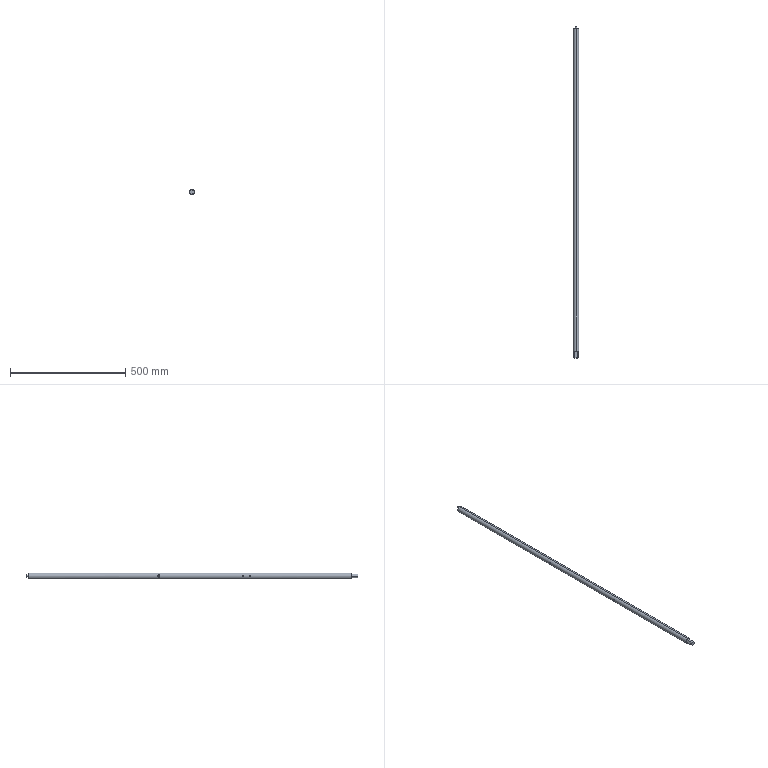Part | SolidWorks | features BaseBody 1 | 1 solid | 29 faces | box 25 x 1442 x 25 mm | volume 693874 mm3 | plane 16 | cylinder 13 | commonest cylinder face diameters 6 x9 10 x2 25 x2
STEP:
#1=CARTESIAN_POINT('',(933.402,-3520.973,899.971));
#2=VERTEX_POINT('',#1);
#3=CARTESIAN_POINT('',(933.402,-3520.973,889.971));
#4=VERTEX_POINT('',#3);
#5=CARTESIAN_POINT('',(933.402,-3520.973,899.971));
#6=CARTESIAN_POINT('',(933.402,-3520.643,899.971));
#7=CARTESIAN_POINT('',(933.417,-3520.308,899.938));
#8=CARTESIAN_POINT('',(933.472,-3519.665,899.808));
#9=CARTESIAN_POINT('',(933.512,-3519.351,899.712));
#10=CARTESIAN_POINT('',(933.613,-3518.743,899.458));
#11=CARTESIAN_POINT('',(933.672,-3518.457,899.304));
#12=CARTESIAN_POINT('',(933.799,-3517.919,898.944));
#13=CARTESIAN_POINT('',(933.868,-3517.665,898.735));
#14=CARTESIAN_POINT('',(934.003,-3517.208,898.277));
#15=CARTESIAN_POINT('',(934.069,-3517.003,898.029));
#16=CARTESIAN_POINT('',(934.193,-3516.641,897.489));
#17=CARTESIAN_POINT('',(934.249,-3516.484,897.198));
#18=CARTESIAN_POINT('',(934.343,-3516.234,896.597));
#19=CARTESIAN_POINT('',(934.381,-3516.137,896.285));
#20=CARTESIAN_POINT('',(934.432,-3516.006,895.634));
#21=CARTESIAN_POINT('',(934.446,-3515.973,895.302));
#22=CARTESIAN_POINT('',(934.445,-3515.973,894.635));
#23=CARTESIAN_POINT('',(934.432,-3516.007,894.307));
#24=CARTESIAN_POINT('',(934.381,-3516.136,893.664));
#25=CARTESIAN_POINT('',(934.343,-3516.234,893.345));
#26=CARTESIAN_POINT('',(934.249,-3516.486,892.741));
#27=CARTESIAN_POINT('',(934.193,-3516.64,892.455));
#28=CARTESIAN_POINT('',(934.069,-3517.003,891.915));
#29=CARTESIAN_POINT('',(934.002,-3517.211,891.662));
#30=CARTESIAN_POINT('',(933.867,-3517.667,891.206));
#31=CARTESIAN_POINT('',(933.8,-3517.917,891.));
#32=CARTESIAN_POINT('',(933.671,-3518.46,890.637));
#33=CARTESIAN_POINT('',(933.613,-3518.745,890.483));
#34=CARTESIAN_POINT('',(933.538,-3519.195,890.295));
#35=CARTESIAN_POINT('',(933.516,-3519.348,890.24));
#36=CARTESIAN_POINT('',(933.476,-3519.663,890.143));
#37=CARTESIAN_POINT('',(933.458,-3519.824,890.102));
#38=CARTESIAN_POINT('',(933.417,-3520.31,890.005));
#39=CARTESIAN_POINT('',(933.402,-3520.639,889.971));
#40=CARTESIAN_POINT('',(933.402,-3520.973,889.971));
#41=B_SPLINE_CURVE_WITH_KNOTS('',3,(#5,#6,#7,#8,#9,#10,#11,#12,#13,#14,#15,#16,#17,#18,#19,#20,#21,#22,#23,#24,#25,#26,#27,#28,#29,#30,#31,#32,#33,#34,#35,#36,#37,#38,#39,#40),.UNSPECIFIED.,.F.,.F.,(4,2,2,2,2,2,2,2,2,2,2,2,2,2,2,2,2,4),(0.02369,0.02468,0.02567,0.02665,0.02764,0.02863,0.02961,0.0306,0.03158,0.03257,0.03356,0.03454,0.03553,0.03652,0.0375,0.038,0.03849,0.03948),.UNSPECIFIED.);
#42=EDGE_CURVE('',#2,#4,#41,.T.);
#43=ORIENTED_EDGE('',*,*,#42,.T.);
#44=CARTESIAN_POINT('',(933.402,-3520.973,889.971));
#45=CARTESIAN_POINT('',(933.402,-3521.307,889.971));
#46=CARTESIAN_POINT('',(933.417,-3521.635,890.005));
#47=CARTESIAN_POINT('',(933.472,-3522.279,890.134));
#48=CARTESIAN_POINT('',(933.513,-3522.598,890.231));
#49=CARTESIAN_POINT('',(933.613,-3523.201,890.483));
#50=CARTESIAN_POINT('',(933.672,-3523.487,890.637));
#51=CARTESIAN_POINT('',(933.799,-3524.028,891.));
#52=CARTESIAN_POINT('',(933.868,-3524.28,891.208));
#53=CARTESIAN_POINT('',(934.002,-3524.737,891.664));
#54=CARTESIAN_POINT('',(934.069,-3524.943,891.914));
#55=CARTESIAN_POINT('',(934.193,-3525.308,892.458));
#56=CARTESIAN_POINT('',(934.249,-3525.461,892.744));
#57=CARTESIAN_POINT('',(934.32,-3525.649,893.194));
#58=CARTESIAN_POINT('',(934.341,-3525.705,893.348));
#59=CARTESIAN_POINT('',(934.378,-3525.802,893.663));
#60=CARTESIAN_POINT('',(934.394,-3525.843,893.825));
#61=CARTESIAN_POINT('',(934.432,-3525.94,894.312));
#62=CARTESIAN_POINT('',(934.446,-3525.973,894.641));
#63=CARTESIAN_POINT('',(934.445,-3525.973,895.309));
#64=CARTESIAN_POINT('',(934.432,-3525.939,895.637));
#65=CARTESIAN_POINT('',(934.381,-3525.81,896.281));
#66=CARTESIAN_POINT('',(934.343,-3525.712,896.6));
#67=CARTESIAN_POINT('',(934.248,-3525.459,897.204));
#68=CARTESIAN_POINT('',(934.192,-3525.305,897.49));
#69=CARTESIAN_POINT('',(934.069,-3524.941,898.031));
#70=CARTESIAN_POINT('',(934.001,-3524.732,898.284));
#71=CARTESIAN_POINT('',(933.867,-3524.276,898.739));
#72=CARTESIAN_POINT('',(933.799,-3524.025,898.945));
#73=CARTESIAN_POINT('',(933.67,-3523.482,899.309));
#74=CARTESIAN_POINT('',(933.612,-3523.196,899.462));
#75=CARTESIAN_POINT('',(933.537,-3522.746,899.65));
#76=CARTESIAN_POINT('',(933.515,-3522.592,899.705));
#77=CARTESIAN_POINT('',(933.475,-3522.277,899.801));
#78=CARTESIAN_POINT('',(933.458,-3522.115,899.842));
#79=CARTESIAN_POINT('',(933.416,-3521.63,899.939));
#80=CARTESIAN_POINT('',(933.402,-3521.303,899.971));
#81=CARTESIAN_POINT('',(933.402,-3520.973,899.971));
#82=B_SPLINE_CURVE_WITH_KNOTS('',3,(#44,#45,#46,#47,#48,#49,#50,#51,#52,#53,#54,#55,#56,#57,#58,#59,#60,#61,#62,#63,#64,#65,#66,#67,#68,#69,#70,#71,#72,#73,#74,#75,#76,#77,#78,#79,#80,#81),.UNSPECIFIED.,.F.,.F.,(4,2,2,2,2,2,2,2,2,2,2,2,2,2,2,2,2,2,4),(0.007895,0.008882,0.00987,0.01086,0.01184,0.01283,0.01382,0.01431,0.01481,0.01579,0.01678,0.01777,0.01876,0.01974,0.02073,0.02172,0.02221,0.02271,0.02369),.UNSPECIFIED.);
#83=EDGE_CURVE('',#4,#2,#82,.T.);
#84=ORIENTED_EDGE('',*,*,#83,.T.);
#85=EDGE_LOOP('',(#43,#84));
#86=FACE_BOUND('',#85,.T.);
#87=CARTESIAN_POINT('',(921.946,-2953.973,882.471));
#88=VERTEX_POINT('',#87);
#89=CARTESIAN_POINT('',(921.946,-2953.973,907.471));
#90=VERTEX_POINT('',#89);
#91=CARTESIAN_POINT('',(921.946,-2953.973,894.971));
#92=DIRECTION('',(0.,-1.,0.));
#93=DIRECTION('',(0.,0.,-1.));
#94=AXIS2_PLACEMENT_3D('',#91,#92,#93);
#95=CIRCLE('',#94,12.5);
#96=EDGE_CURVE('',#88,#90,#95,.T.);
#97=ORIENTED_EDGE('',*,*,#96,.T.);
#98=CARTESIAN_POINT('',(921.946,-4355.973,907.471));
#99=VERTEX_POINT('',#98);
#100=CARTESIAN_POINT('',(921.946,-3669.973,907.471));
#101=DIRECTION('',(0.,-1.,0.));
#102=VECTOR('',#101,1000.);
#103=LINE('',#100,#102);
#104=EDGE_CURVE('',#90,#99,#103,.T.);
#105=ORIENTED_EDGE('',*,*,#104,.T.);
#106=CARTESIAN_POINT('',(921.946,-4355.973,882.471));
#107=VERTEX_POINT('',#106);
#108=CARTESIAN_POINT('',(921.946,-4355.973,894.971));
#109=DIRECTION('',(0.,1.,0.));
#110=DIRECTION('',(0.,0.,-1.));
#111=AXIS2_PLACEMENT_3D('',#108,#109,#110);
#112=CIRCLE('',#111,12.5);
#113=EDGE_CURVE('',#99,#107,#112,.T.);
#114=ORIENTED_EDGE('',*,*,#113,.T.);
#115=CARTESIAN_POINT('',(921.946,-3669.973,882.471));
#116=DIRECTION('',(0.,-1.,0.));
#117=VECTOR('',#116,1000.);
#118=LINE('',#115,#117);
#119=EDGE_CURVE('',#88,#107,#118,.T.);
#120=ORIENTED_EDGE('',*,*,#119,.F.);
#121=EDGE_LOOP('',(#97,#105,#114,#120));
#122=FACE_OUTER_BOUND('',#121,.T.);
#123=CARTESIAN_POINT('',(921.946,-3669.973,894.971));
#124=DIRECTION('',(0.,-1.,0.));
#125=DIRECTION('',(0.,0.,-1.));
#126=AXIS2_PLACEMENT_3D('',#123,#124,#125);
#127=CYLINDRICAL_SURFACE('',#126,12.5);
#128=ADVANCED_FACE('',(#86,#122),#127,.T.);
#129=ORIENTED_EDGE('',*,*,#83,.F.);
#130=CARTESIAN_POINT('',(910.489,-3520.973,889.971));
#131=VERTEX_POINT('',#130);
#132=CARTESIAN_POINT('',(921.679,-3520.973,889.971));
#133=DIRECTION('',(-1.,0.,0.));
#134=VECTOR('',#133,1000.);
#135=LINE('',#132,#134);
#136=EDGE_CURVE('',#4,#131,#135,.T.);
#137=ORIENTED_EDGE('',*,*,#136,.T.);
#138=CARTESIAN_POINT('',(910.489,-3520.973,899.971));
#139=VERTEX_POINT('',#138);
#140=CARTESIAN_POINT('',(910.489,-3520.973,899.971));
#141=CARTESIAN_POINT('',(910.489,-3521.303,899.971));
#142=CARTESIAN_POINT('',(910.474,-3521.638,899.938));
#143=CARTESIAN_POINT('',(910.419,-3522.282,899.808));
#144=CARTESIAN_POINT('',(910.379,-3522.595,899.712));
#145=CARTESIAN_POINT('',(910.278,-3523.204,899.458));
#146=CARTESIAN_POINT('',(910.219,-3523.489,899.304));
#147=CARTESIAN_POINT('',(910.092,-3524.027,898.944));
#148=CARTESIAN_POINT('',(910.023,-3524.281,898.735));
#149=CARTESIAN_POINT('',(909.888,-3524.738,898.277));
#150=CARTESIAN_POINT('',(909.822,-3524.943,898.029));
#151=CARTESIAN_POINT('',(909.699,-3525.305,897.489));
#152=CARTESIAN_POINT('',(909.642,-3525.462,897.198));
#153=CARTESIAN_POINT('',(909.548,-3525.713,896.597));
#154=CARTESIAN_POINT('',(909.51,-3525.809,896.285));
#155=CARTESIAN_POINT('',(909.459,-3525.94,895.634));
#156=CARTESIAN_POINT('',(909.445,-3525.973,895.302));
#157=CARTESIAN_POINT('',(909.446,-3525.973,894.635));
#158=CARTESIAN_POINT('',(909.459,-3525.94,894.307));
#159=CARTESIAN_POINT('',(909.51,-3525.81,893.664));
#160=CARTESIAN_POINT('',(909.548,-3525.712,893.345));
#161=CARTESIAN_POINT('',(909.642,-3525.46,892.741));
#162=CARTESIAN_POINT('',(909.698,-3525.306,892.455));
#163=CARTESIAN_POINT('',(909.822,-3524.943,891.915));
#164=CARTESIAN_POINT('',(909.889,-3524.735,891.662));
#165=CARTESIAN_POINT('',(910.024,-3524.279,891.206));
#166=CARTESIAN_POINT('',(910.092,-3524.029,891.));
#167=CARTESIAN_POINT('',(910.22,-3523.486,890.637));
#168=CARTESIAN_POINT('',(910.278,-3523.201,890.483));
#169=CARTESIAN_POINT('',(910.353,-3522.751,890.295));
#170=CARTESIAN_POINT('',(910.376,-3522.598,890.24));
#171=CARTESIAN_POINT('',(910.415,-3522.283,890.143));
#172=CARTESIAN_POINT('',(910.433,-3522.122,890.102));
#173=CARTESIAN_POINT('',(910.474,-3521.636,890.005));
#174=CARTESIAN_POINT('',(910.489,-3521.307,889.971));
#175=CARTESIAN_POINT('',(910.489,-3520.973,889.971));
#176=B_SPLINE_CURVE_WITH_KNOTS('',3,(#140,#141,#142,#143,#144,#145,#146,#147,#148,#149,#150,#151,#152,#153,#154,#155,#156,#157,#158,#159,#160,#161,#162,#163,#164,#165,#166,#167,#168,#169,#170,#171,#172,#173,#174,#175),.UNSPECIFIED.,.F.,.F.,(4,2,2,2,2,2,2,2,2,2,2,2,2,2,2,2,2,4),(0.02369,0.02468,0.02567,0.02665,0.02764,0.02863,0.02961,0.0306,0.03158,0.03257,0.03356,0.03454,0.03553,0.03652,0.0375,0.038,0.03849,0.03948),.UNSPECIFIED.);
#177=EDGE_CURVE('',#139,#131,#176,.T.);
#178=ORIENTED_EDGE('',*,*,#177,.F.);
#179=CARTESIAN_POINT('',(921.679,-3520.973,899.971));
#180=DIRECTION('',(-1.,0.,0.));
#181=VECTOR('',#180,1000.);
#182=LINE('',#179,#181);
#183=EDGE_CURVE('',#2,#139,#182,.T.);
#184=ORIENTED_EDGE('',*,*,#183,.F.);
#185=EDGE_LOOP('',(#129,#137,#178,#184));
#186=FACE_OUTER_BOUND('',#185,.T.);
#187=CARTESIAN_POINT('',(921.679,-3520.973,894.971));
#188=DIRECTION('',(-1.,0.,0.));
#189=DIRECTION('',(0.,0.,1.));
#190=AXIS2_PLACEMENT_3D('',#187,#188,#189);
#191=CYLINDRICAL_SURFACE('',#190,5.);
#192=ADVANCED_FACE('',(#186),#191,.F.);
#193=CARTESIAN_POINT('',(916.446,-3885.973,892.044));
#194=VERTEX_POINT('',#193);
#195=CARTESIAN_POINT('',(916.446,-3885.973,898.044));
#196=VERTEX_POINT('',#195);
#197=CARTESIAN_POINT('',(916.446,-3885.973,895.044));
#198=DIRECTION('',(-1.,0.,0.));
#199=DIRECTION('',(0.,0.,1.));
#200=AXIS2_PLACEMENT_3D('',#197,#198,#199);
#201=CIRCLE('',#200,3.);
#202=EDGE_CURVE('',#194,#196,#201,.T.);
#203=ORIENTED_EDGE('',*,*,#202,.F.);
#204=CARTESIAN_POINT('',(909.793,-3885.973,892.044));
#205=VERTEX_POINT('',#204);
#206=CARTESIAN_POINT('',(866.446,-3885.973,892.044));
#207=DIRECTION('',(-1.,0.,0.));
#208=VECTOR('',#207,1000.);
#209=LINE('',#206,#208);
#210=EDGE_CURVE('',#194,#205,#209,.T.);
#211=ORIENTED_EDGE('',*,*,#210,.T.);
#212=CARTESIAN_POINT('',(909.829,-3885.973,898.044));
#213=VERTEX_POINT('',#212);
#214=CARTESIAN_POINT('',(909.829,-3885.973,898.044));
#215=CARTESIAN_POINT('',(909.829,-3886.169,898.044));
#216=CARTESIAN_POINT('',(909.824,-3886.369,898.024));
#217=CARTESIAN_POINT('',(909.805,-3886.754,897.947));
#218=CARTESIAN_POINT('',(909.791,-3886.941,897.89));
#219=CARTESIAN_POINT('',(909.738,-3887.487,897.664));
#220=CARTESIAN_POINT('',(909.689,-3887.816,897.443));
#221=CARTESIAN_POINT('',(909.615,-3888.233,897.027));
#222=CARTESIAN_POINT('',(909.59,-3888.356,896.877));
#223=CARTESIAN_POINT('',(909.545,-3888.573,896.553));
#224=CARTESIAN_POINT('',(909.524,-3888.668,896.377));
#225=CARTESIAN_POINT('',(909.488,-3888.818,896.016));
#226=CARTESIAN_POINT('',(909.473,-3888.875,895.829));
#227=CARTESIAN_POINT('',(909.453,-3888.953,895.443));
#228=CARTESIAN_POINT('',(909.447,-3888.973,895.244));
#229=CARTESIAN_POINT('',(909.445,-3888.973,894.847));
#230=CARTESIAN_POINT('',(909.448,-3888.954,894.65));
#231=CARTESIAN_POINT('',(909.464,-3888.877,894.266));
#232=CARTESIAN_POINT('',(909.476,-3888.82,894.076));
#233=CARTESIAN_POINT('',(909.508,-3888.669,893.712));
#234=CARTESIAN_POINT('',(909.527,-3888.576,893.54));
#235=CARTESIAN_POINT('',(909.568,-3888.359,893.215));
#236=CARTESIAN_POINT('',(909.592,-3888.233,893.061));
#237=CARTESIAN_POINT('',(909.637,-3887.957,892.785));
#238=CARTESIAN_POINT('',(909.66,-3887.807,892.661));
#239=CARTESIAN_POINT('',(909.703,-3887.481,892.443));
#240=CARTESIAN_POINT('',(909.723,-3887.306,892.349));
#241=CARTESIAN_POINT('',(909.773,-3886.765,892.124));
#242=CARTESIAN_POINT('',(909.793,-3886.371,892.044));
#243=CARTESIAN_POINT('',(909.793,-3885.973,892.044));
#244=B_SPLINE_CURVE_WITH_KNOTS('',3,(#214,#215,#216,#217,#218,#219,#220,#221,#222,#223,#224,#225,#226,#227,#228,#229,#230,#231,#232,#233,#234,#235,#236,#237,#238,#239,#240,#241,#242,#243),.UNSPECIFIED.,.F.,.F.,(4,2,2,2,2,2,2,2,2,2,2,2,2,2,4),(0.01404,0.01463,0.01522,0.01639,0.01698,0.01757,0.01816,0.01874,0.01933,0.01992,0.02051,0.0211,0.02168,0.02227,0.02345),.UNSPECIFIED.);
#245=EDGE_CURVE('',#213,#205,#244,.T.);
#246=ORIENTED_EDGE('',*,*,#245,.F.);
#247=CARTESIAN_POINT('',(866.446,-3885.973,898.044));
#248=DIRECTION('',(-1.,0.,0.));
#249=VECTOR('',#248,1000.);
#250=LINE('',#247,#249);
#251=EDGE_CURVE('',#196,#213,#250,.T.);
#252=ORIENTED_EDGE('',*,*,#251,.F.);
#253=EDGE_LOOP('',(#203,#211,#246,#252));
#254=FACE_OUTER_BOUND('',#253,.T.);
#255=CARTESIAN_POINT('',(866.446,-3885.973,895.044));
#256=DIRECTION('',(-1.,0.,0.));
#257=DIRECTION('',(0.,0.,1.));
#258=AXIS2_PLACEMENT_3D('',#255,#256,#257);
#259=CYLINDRICAL_SURFACE('',#258,3.);
#260=ADVANCED_FACE('',(#254),#259,.F.);
#261=CARTESIAN_POINT('',(916.446,-3915.973,892.044));
#262=VERTEX_POINT('',#261);
#263=CARTESIAN_POINT('',(916.446,-3915.973,898.044));
#264=VERTEX_POINT('',#263);
#265=CARTESIAN_POINT('',(916.446,-3915.973,895.044));
#266=DIRECTION('',(-1.,0.,0.));
#267=DIRECTION('',(0.,0.,1.));
#268=AXIS2_PLACEMENT_3D('',#265,#266,#267);
#269=CIRCLE('',#268,3.);
#270=EDGE_CURVE('',#262,#264,#269,.T.);
#271=ORIENTED_EDGE('',*,*,#270,.F.);
#272=CARTESIAN_POINT('',(909.793,-3915.973,892.044));
#273=VERTEX_POINT('',#272);
#274=CARTESIAN_POINT('',(866.446,-3915.973,892.044));
#275=DIRECTION('',(-1.,0.,0.));
#276=VECTOR('',#275,1000.);
#277=LINE('',#274,#276);
#278=EDGE_CURVE('',#262,#273,#277,.T.);
#279=ORIENTED_EDGE('',*,*,#278,.T.);
#280=CARTESIAN_POINT('',(909.829,-3915.973,898.044));
#281=VERTEX_POINT('',#280);
#282=CARTESIAN_POINT('',(909.829,-3915.973,898.044));
#283=CARTESIAN_POINT('',(909.829,-3916.169,898.044));
#284=CARTESIAN_POINT('',(909.824,-3916.369,898.024));
#285=CARTESIAN_POINT('',(909.805,-3916.754,897.947));
#286=CARTESIAN_POINT('',(909.791,-3916.941,897.89));
#287=CARTESIAN_POINT('',(909.738,-3917.487,897.664));
#288=CARTESIAN_POINT('',(909.689,-3917.816,897.443));
#289=CARTESIAN_POINT('',(909.615,-3918.233,897.027));
#290=CARTESIAN_POINT('',(909.59,-3918.356,896.877));
#291=CARTESIAN_POINT('',(909.545,-3918.573,896.553));
#292=CARTESIAN_POINT('',(909.524,-3918.668,896.377));
#293=CARTESIAN_POINT('',(909.488,-3918.818,896.016));
#294=CARTESIAN_POINT('',(909.473,-3918.875,895.829));
#295=CARTESIAN_POINT('',(909.453,-3918.953,895.443));
#296=CARTESIAN_POINT('',(909.447,-3918.973,895.244));
#297=CARTESIAN_POINT('',(909.445,-3918.973,894.847));
#298=CARTESIAN_POINT('',(909.448,-3918.954,894.65));
#299=CARTESIAN_POINT('',(909.464,-3918.877,894.266));
#300=CARTESIAN_POINT('',(909.476,-3918.82,894.076));
#301=CARTESIAN_POINT('',(909.508,-3918.669,893.712));
#302=CARTESIAN_POINT('',(909.527,-3918.576,893.54));
#303=CARTESIAN_POINT('',(909.568,-3918.359,893.215));
#304=CARTESIAN_POINT('',(909.592,-3918.233,893.061));
#305=CARTESIAN_POINT('',(909.637,-3917.957,892.785));
#306=CARTESIAN_POINT('',(909.66,-3917.807,892.661));
#307=CARTESIAN_POINT('',(909.703,-3917.481,892.443));
#308=CARTESIAN_POINT('',(909.723,-3917.306,892.349));
#309=CARTESIAN_POINT('',(909.773,-3916.765,892.124));
#310=CARTESIAN_POINT('',(909.793,-3916.371,892.044));
#311=CARTESIAN_POINT('',(909.793,-3915.973,892.044));
#312=B_SPLINE_CURVE_WITH_KNOTS('',3,(#282,#283,#284,#285,#286,#287,#288,#289,#290,#291,#292,#293,#294,#295,#296,#297,#298,#299,#300,#301,#302,#303,#304,#305,#306,#307,#308,#309,#310,#311),.UNSPECIFIED.,.F.,.F.,(4,2,2,2,2,2,2,2,2,2,2,2,2,2,4),(0.01404,0.01463,0.01522,0.01639,0.01698,0.01757,0.01816,0.01874,0.01933,0.01992,0.02051,0.0211,0.02168,0.02227,0.02345),.UNSPECIFIED.);
#313=EDGE_CURVE('',#281,#273,#312,.T.);
#314=ORIENTED_EDGE('',*,*,#313,.F.);
#315=CARTESIAN_POINT('',(866.446,-3915.973,898.044));
#316=DIRECTION('',(-1.,0.,0.));
#317=VECTOR('',#316,1000.);
#318=LINE('',#315,#317);
#319=EDGE_CURVE('',#264,#281,#318,.T.);
#320=ORIENTED_EDGE('',*,*,#319,.F.);
#321=EDGE_LOOP('',(#271,#279,#314,#320));
#322=FACE_OUTER_BOUND('',#321,.T.);
#323=CARTESIAN_POINT('',(866.446,-3915.973,895.044));
#324=DIRECTION('',(-1.,0.,0.));
#325=DIRECTION('',(0.,0.,1.));
#326=AXIS2_PLACEMENT_3D('',#323,#324,#325);
#327=CYLINDRICAL_SURFACE('',#326,3.);
#328=ADVANCED_FACE('',(#322),#327,.F.);
#329=CARTESIAN_POINT('',(921.946,-2953.973,891.971));
#330=VERTEX_POINT('',#329);
#331=CARTESIAN_POINT('',(921.946,-2953.973,897.971));
#332=VERTEX_POINT('',#331);
#333=CARTESIAN_POINT('',(921.946,-2953.973,894.971));
#334=DIRECTION('',(0.,-1.,0.));
#335=DIRECTION('',(0.,0.,1.));
#336=AXIS2_PLACEMENT_3D('',#333,#334,#335);
#337=CIRCLE('',#336,3.);
#338=EDGE_CURVE('',#330,#332,#337,.T.);
#339=ORIENTED_EDGE('',*,*,#338,.F.);
#340=CARTESIAN_POINT('',(921.946,-2947.973,891.971));
#341=VERTEX_POINT('',#340);
#342=CARTESIAN_POINT('',(921.946,-2952.973,891.971));
#343=DIRECTION('',(0.,1.,0.));
#344=VECTOR('',#343,1000.);
#345=LINE('',#342,#344);
#346=EDGE_CURVE('',#330,#341,#345,.T.);
#347=ORIENTED_EDGE('',*,*,#346,.T.);
#348=CARTESIAN_POINT('',(924.946,-2947.973,894.971));
#349=VERTEX_POINT('',#348);
#350=CARTESIAN_POINT('',(921.946,-2947.973,894.971));
#351=DIRECTION('',(0.,-1.,0.));
#352=DIRECTION('',(0.,0.,1.));
#353=AXIS2_PLACEMENT_3D('',#350,#351,#352);
#354=CIRCLE('',#353,3.);
#355=EDGE_CURVE('',#341,#349,#354,.T.);
#356=ORIENTED_EDGE('',*,*,#355,.T.);
#357=CARTESIAN_POINT('',(921.946,-2947.973,897.971));
#358=VERTEX_POINT('',#357);
#359=CARTESIAN_POINT('',(921.946,-2947.973,894.971));
#360=DIRECTION('',(0.,-1.,0.));
#361=DIRECTION('',(0.,0.,1.));
#362=AXIS2_PLACEMENT_3D('',#359,#360,#361);
#363=CIRCLE('',#362,3.);
#364=EDGE_CURVE('',#349,#358,#363,.T.);
#365=ORIENTED_EDGE('',*,*,#364,.T.);
#366=CARTESIAN_POINT('',(921.946,-2952.973,897.971));
#367=DIRECTION('',(0.,1.,0.));
#368=VECTOR('',#367,1000.);
#369=LINE('',#366,#368);
#370=EDGE_CURVE('',#332,#358,#369,.T.);
#371=ORIENTED_EDGE('',*,*,#370,.F.);
#372=EDGE_LOOP('',(#339,#347,#356,#365,#371));
#373=FACE_OUTER_BOUND('',#372,.T.);
#374=CARTESIAN_POINT('',(921.946,-2952.973,894.971));
#375=DIRECTION('',(0.,1.,0.));
#376=DIRECTION('',(0.,0.,1.));
#377=AXIS2_PLACEMENT_3D('',#374,#375,#376);
#378=CYLINDRICAL_SURFACE('',#377,3.);
#379=ADVANCED_FACE('',(#373),#378,.T.);
#380=CARTESIAN_POINT('',(918.946,-2947.973,898.971));
#381=VERTEX_POINT('',#380);
#382=CARTESIAN_POINT('',(921.946,-2947.973,901.971));
#383=VERTEX_POINT('',#382);
#384=CARTESIAN_POINT('',(921.946,-2947.973,898.971));
#385=DIRECTION('',(0.,1.,0.));
#386=DIRECTION('',(0.,0.,1.));
#387=AXIS2_PLACEMENT_3D('',#384,#385,#386);
#388=CIRCLE('',#387,3.);
#389=EDGE_CURVE('',#381,#383,#388,.T.);
#390=ORIENTED_EDGE('',*,*,#389,.T.);
#391=CARTESIAN_POINT('',(921.946,-2943.973,901.971));
#392=VERTEX_POINT('',#391);
#393=CARTESIAN_POINT('',(921.946,-2947.973,901.971));
#394=DIRECTION('',(0.,1.,0.));
#395=VECTOR('',#394,1000.);
#396=LINE('',#393,#395);
#397=EDGE_CURVE('',#383,#392,#396,.T.);
#398=ORIENTED_EDGE('',*,*,#397,.T.);
#399=CARTESIAN_POINT('',(918.946,-2943.973,898.971));
#400=VERTEX_POINT('',#399);
#401=CARTESIAN_POINT('',(921.946,-2943.973,898.971));
#402=DIRECTION('',(0.,-1.,0.));
#403=DIRECTION('',(0.,0.,1.));
#404=AXIS2_PLACEMENT_3D('',#401,#402,#403);
#405=CIRCLE('',#404,3.);
#406=EDGE_CURVE('',#392,#400,#405,.T.);
#407=ORIENTED_EDGE('',*,*,#406,.T.);
#408=CARTESIAN_POINT('',(918.946,-2947.973,898.971));
#409=DIRECTION('',(0.,-1.,0.));
#410=VECTOR('',#409,1000.);
#411=LINE('',#408,#410);
#412=EDGE_CURVE('',#400,#381,#411,.T.);
#413=ORIENTED_EDGE('',*,*,#412,.T.);
#414=EDGE_LOOP('',(#390,#398,#407,#413));
#415=FACE_OUTER_BOUND('',#414,.T.);
#416=CARTESIAN_POINT('',(921.946,-2947.973,898.971));
#417=DIRECTION('',(0.,1.,0.));
#418=DIRECTION('',(0.,0.,1.));
#419=AXIS2_PLACEMENT_3D('',#416,#417,#418);
#420=CYLINDRICAL_SURFACE('',#419,3.);
#421=ADVANCED_FACE('',(#415),#420,.T.);
#422=ORIENTED_EDGE('',*,*,#104,.F.);
#423=CARTESIAN_POINT('',(921.946,-2953.973,894.971));
#424=DIRECTION('',(0.,-1.,0.));
#425=DIRECTION('',(0.,0.,-1.));
#426=AXIS2_PLACEMENT_3D('',#423,#424,#425);
#427=CIRCLE('',#426,12.5);
#428=EDGE_CURVE('',#90,#88,#427,.T.);
#429=ORIENTED_EDGE('',*,*,#428,.T.);
#430=ORIENTED_EDGE('',*,*,#119,.T.);
#431=CARTESIAN_POINT('',(921.946,-4355.973,894.971));
#432=DIRECTION('',(0.,1.,0.));
#433=DIRECTION('',(0.,0.,-1.));
#434=AXIS2_PLACEMENT_3D('',#431,#432,#433);
#435=CIRCLE('',#434,12.5);
#436=EDGE_CURVE('',#107,#99,#435,.T.);
#437=ORIENTED_EDGE('',*,*,#436,.T.);
#438=EDGE_LOOP('',(#422,#429,#430,#437));
#439=FACE_OUTER_BOUND('',#438,.T.);
#440=ORIENTED_EDGE('',*,*,#313,.T.);
#441=CARTESIAN_POINT('',(909.793,-3915.973,892.044));
#442=CARTESIAN_POINT('',(909.793,-3915.774,892.044));
#443=CARTESIAN_POINT('',(909.788,-3915.579,892.064));
#444=CARTESIAN_POINT('',(909.77,-3915.194,892.14));
#445=CARTESIAN_POINT('',(909.757,-3915.003,892.198));
#446=CARTESIAN_POINT('',(909.723,-3914.64,892.349));
#447=CARTESIAN_POINT('',(909.704,-3914.468,892.441));
#448=CARTESIAN_POINT('',(909.661,-3914.143,892.659));
#449=CARTESIAN_POINT('',(909.637,-3913.989,892.785));
#450=CARTESIAN_POINT('',(909.592,-3913.714,893.061));
#451=CARTESIAN_POINT('',(909.569,-3913.59,893.211));
#452=CARTESIAN_POINT('',(909.527,-3913.37,893.539));
#453=CARTESIAN_POINT('',(909.508,-3913.277,893.713));
#454=CARTESIAN_POINT('',(909.461,-3913.053,894.254));
#455=CARTESIAN_POINT('',(909.443,-3912.973,894.65));
#456=CARTESIAN_POINT('',(909.447,-3912.973,895.247));
#457=CARTESIAN_POINT('',(909.453,-3912.993,895.442));
#458=CARTESIAN_POINT('',(909.473,-3913.07,895.827));
#459=CARTESIAN_POINT('',(909.488,-3913.129,896.017));
#460=CARTESIAN_POINT('',(909.524,-3913.28,896.38));
#461=CARTESIAN_POINT('',(909.545,-3913.372,896.552));
#462=CARTESIAN_POINT('',(909.591,-3913.59,896.877));
#463=CARTESIAN_POINT('',(909.615,-3913.716,897.03));
#464=CARTESIAN_POINT('',(909.665,-3913.992,897.305));
#465=CARTESIAN_POINT('',(909.689,-3914.143,897.429));
#466=CARTESIAN_POINT('',(909.735,-3914.47,897.648));
#467=CARTESIAN_POINT('',(909.756,-3914.644,897.74));
#468=CARTESIAN_POINT('',(909.791,-3915.004,897.89));
#469=CARTESIAN_POINT('',(909.805,-3915.194,897.948));
#470=CARTESIAN_POINT('',(909.824,-3915.582,898.025));
#471=CARTESIAN_POINT('',(909.829,-3915.777,898.044));
#472=CARTESIAN_POINT('',(909.829,-3915.973,898.044));
#473=B_SPLINE_CURVE_WITH_KNOTS('',3,(#441,#442,#443,#444,#445,#446,#447,#448,#449,#450,#451,#452,#453,#454,#455,#456,#457,#458,#459,#460,#461,#462,#463,#464,#465,#466,#467,#468,#469,#470,#471,#472),.UNSPECIFIED.,.F.,.F.,(4,2,2,2,2,2,2,2,2,2,2,2,2,2,2,4),(0.00463,0.005218,0.005806,0.006395,0.006983,0.007571,0.008159,0.009336,0.009924,0.01051,0.0111,0.01169,0.01228,0.01286,0.01345,0.01404),.UNSPECIFIED.);
#474=EDGE_CURVE('',#273,#281,#473,.T.);
#475=ORIENTED_EDGE('',*,*,#474,.T.);
#476=EDGE_LOOP('',(#440,#475));
#477=FACE_BOUND('',#476,.T.);
#478=ORIENTED_EDGE('',*,*,#245,.T.);
#479=CARTESIAN_POINT('',(909.793,-3885.973,892.044));
#480=CARTESIAN_POINT('',(909.793,-3885.774,892.044));
#481=CARTESIAN_POINT('',(909.788,-3885.579,892.064));
#482=CARTESIAN_POINT('',(909.77,-3885.194,892.14));
#483=CARTESIAN_POINT('',(909.757,-3885.003,892.198));
#484=CARTESIAN_POINT('',(909.723,-3884.64,892.349));
#485=CARTESIAN_POINT('',(909.704,-3884.468,892.441));
#486=CARTESIAN_POINT('',(909.661,-3884.143,892.659));
#487=CARTESIAN_POINT('',(909.637,-3883.989,892.785));
#488=CARTESIAN_POINT('',(909.592,-3883.714,893.061));
#489=CARTESIAN_POINT('',(909.569,-3883.59,893.211));
#490=CARTESIAN_POINT('',(909.527,-3883.37,893.539));
#491=CARTESIAN_POINT('',(909.508,-3883.277,893.713));
#492=CARTESIAN_POINT('',(909.461,-3883.053,894.254));
#493=CARTESIAN_POINT('',(909.443,-3882.973,894.65));
#494=CARTESIAN_POINT('',(909.447,-3882.973,895.247));
#495=CARTESIAN_POINT('',(909.453,-3882.993,895.442));
#496=CARTESIAN_POINT('',(909.473,-3883.07,895.827));
#497=CARTESIAN_POINT('',(909.488,-3883.129,896.017));
#498=CARTESIAN_POINT('',(909.524,-3883.28,896.38));
#499=CARTESIAN_POINT('',(909.545,-3883.372,896.552));
#500=CARTESIAN_POINT('',(909.591,-3883.59,896.877));
#501=CARTESIAN_POINT('',(909.615,-3883.716,897.03));
#502=CARTESIAN_POINT('',(909.665,-3883.992,897.305));
#503=CARTESIAN_POINT('',(909.689,-3884.143,897.429));
#504=CARTESIAN_POINT('',(909.735,-3884.47,897.648));
#505=CARTESIAN_POINT('',(909.756,-3884.644,897.74));
#506=CARTESIAN_POINT('',(909.791,-3885.004,897.89));
#507=CARTESIAN_POINT('',(909.805,-3885.194,897.948));
#508=CARTESIAN_POINT('',(909.824,-3885.582,898.025));
#509=CARTESIAN_POINT('',(909.829,-3885.777,898.044));
#510=CARTESIAN_POINT('',(909.829,-3885.973,898.044));
#511=B_SPLINE_CURVE_WITH_KNOTS('',3,(#479,#480,#481,#482,#483,#484,#485,#486,#487,#488,#489,#490,#491,#492,#493,#494,#495,#496,#497,#498,#499,#500,#501,#502,#503,#504,#505,#506,#507,#508,#509,#510),.UNSPECIFIED.,.F.,.F.,(4,2,2,2,2,2,2,2,2,2,2,2,2,2,2,4),(0.00463,0.005218,0.005806,0.006395,0.006983,0.007571,0.008159,0.009336,0.009924,0.01051,0.0111,0.01169,0.01228,0.01286,0.01345,0.01404),.UNSPECIFIED.);
#512=EDGE_CURVE('',#205,#213,#511,.T.);
#513=ORIENTED_EDGE('',*,*,#512,.T.);
#514=EDGE_LOOP('',(#478,#513));
#515=FACE_BOUND('',#514,.T.);
#516=ORIENTED_EDGE('',*,*,#177,.T.);
#517=CARTESIAN_POINT('',(910.489,-3520.973,889.971));
#518=CARTESIAN_POINT('',(910.489,-3520.639,889.971));
#519=CARTESIAN_POINT('',(910.474,-3520.311,890.005));
#520=CARTESIAN_POINT('',(910.419,-3519.668,890.134));
#521=CARTESIAN_POINT('',(910.378,-3519.348,890.231));
#522=CARTESIAN_POINT('',(910.278,-3518.745,890.483));
#523=CARTESIAN_POINT('',(910.219,-3518.459,890.637));
#524=CARTESIAN_POINT('',(910.092,-3517.919,891.));
#525=CARTESIAN_POINT('',(910.023,-3517.666,891.208));
#526=CARTESIAN_POINT('',(909.889,-3517.21,891.664));
#527=CARTESIAN_POINT('',(909.822,-3517.003,891.914));
#528=CARTESIAN_POINT('',(909.698,-3516.638,892.458));
#529=CARTESIAN_POINT('',(909.642,-3516.485,892.744));
#530=CARTESIAN_POINT('',(909.572,-3516.297,893.194));
#531=CARTESIAN_POINT('',(909.55,-3516.241,893.348));
#532=CARTESIAN_POINT('',(909.513,-3516.144,893.663));
#533=CARTESIAN_POINT('',(909.497,-3516.104,893.825));
#534=CARTESIAN_POINT('',(909.459,-3516.006,894.312));
#535=CARTESIAN_POINT('',(909.445,-3515.973,894.641));
#536=CARTESIAN_POINT('',(909.446,-3515.973,895.309));
#537=CARTESIAN_POINT('',(909.459,-3516.007,895.637));
#538=CARTESIAN_POINT('',(909.51,-3516.136,896.281));
#539=CARTESIAN_POINT('',(909.548,-3516.235,896.6));
#540=CARTESIAN_POINT('',(909.643,-3516.487,897.204));
#541=CARTESIAN_POINT('',(909.699,-3516.642,897.49));
#542=CARTESIAN_POINT('',(909.823,-3517.005,898.031));
#543=CARTESIAN_POINT('',(909.89,-3517.214,898.284));
#544=CARTESIAN_POINT('',(910.025,-3517.671,898.739));
#545=CARTESIAN_POINT('',(910.092,-3517.921,898.945));
#546=CARTESIAN_POINT('',(910.221,-3518.465,899.309));
#547=CARTESIAN_POINT('',(910.279,-3518.75,899.462));
#548=CARTESIAN_POINT('',(910.354,-3519.201,899.65));
#549=CARTESIAN_POINT('',(910.376,-3519.354,899.705));
#550=CARTESIAN_POINT('',(910.416,-3519.669,899.801));
#551=CARTESIAN_POINT('',(910.433,-3519.831,899.842));
#552=CARTESIAN_POINT('',(910.475,-3520.316,899.939));
#553=CARTESIAN_POINT('',(910.489,-3520.643,899.971));
#554=CARTESIAN_POINT('',(910.489,-3520.973,899.971));
#555=B_SPLINE_CURVE_WITH_KNOTS('',3,(#517,#518,#519,#520,#521,#522,#523,#524,#525,#526,#527,#528,#529,#530,#531,#532,#533,#534,#535,#536,#537,#538,#539,#540,#541,#542,#543,#544,#545,#546,#547,#548,#549,#550,#551,#552,#553,#554),.UNSPECIFIED.,.F.,.F.,(4,2,2,2,2,2,2,2,2,2,2,2,2,2,2,2,2,2,4),(0.007895,0.008882,0.00987,0.01086,0.01184,0.01283,0.01382,0.01431,0.01481,0.01579,0.01678,0.01777,0.01876,0.01974,0.02073,0.02172,0.02221,0.02271,0.02369),.UNSPECIFIED.);
#556=EDGE_CURVE('',#131,#139,#555,.T.);
#557=ORIENTED_EDGE('',*,*,#556,.T.);
#558=EDGE_LOOP('',(#516,#557));
#559=FACE_BOUND('',#558,.T.);
#560=CARTESIAN_POINT('',(921.946,-3669.973,894.971));
#561=DIRECTION('',(0.,-1.,0.));
#562=DIRECTION('',(0.,0.,-1.));
#563=AXIS2_PLACEMENT_3D('',#560,#561,#562);
#564=CYLINDRICAL_SURFACE('',#563,12.5);
#565=ADVANCED_FACE('',(#439,#477,#515,#559),#564,.T.);
#566=CARTESIAN_POINT('',(921.946,-2953.973,894.971));
#567=DIRECTION('',(0.,-1.,0.));
#568=DIRECTION('',(0.,0.,1.));
#569=AXIS2_PLACEMENT_3D('',#566,#567,#568);
#570=CIRCLE('',#569,3.);
#571=EDGE_CURVE('',#332,#330,#570,.T.);
#572=ORIENTED_EDGE('',*,*,#571,.T.);
#573=ORIENTED_EDGE('',*,*,#338,.T.);
#574=EDGE_LOOP('',(#572,#573));
#575=FACE_BOUND('',#574,.T.);
#576=ORIENTED_EDGE('',*,*,#96,.F.);
#577=ORIENTED_EDGE('',*,*,#428,.F.);
#578=EDGE_LOOP('',(#576,#577));
#579=FACE_OUTER_BOUND('',#578,.T.);
#580=CARTESIAN_POINT('',(921.946,-2953.973,894.971));
#581=DIRECTION('',(0.,1.,0.));
#582=DIRECTION('',(0.,0.,1.));
#583=AXIS2_PLACEMENT_3D('',#580,#581,#582);
#584=PLANE('',#583);
#585=ADVANCED_FACE('',(#575,#579),#584,.T.);
#586=ORIENTED_EDGE('',*,*,#136,.F.);
#587=ORIENTED_EDGE('',*,*,#42,.F.);
#588=ORIENTED_EDGE('',*,*,#183,.T.);
#589=ORIENTED_EDGE('',*,*,#556,.F.);
#590=EDGE_LOOP('',(#586,#587,#588,#589));
#591=FACE_OUTER_BOUND('',#590,.T.);
#592=CARTESIAN_POINT('',(921.679,-3520.973,894.971));
#593=DIRECTION('',(-1.,0.,0.));
#594=DIRECTION('',(0.,0.,1.));
#595=AXIS2_PLACEMENT_3D('',#592,#593,#594);
#596=CYLINDRICAL_SURFACE('',#595,5.);
#597=ADVANCED_FACE('',(#591),#596,.F.);
#598=ORIENTED_EDGE('',*,*,#210,.F.);
#599=CARTESIAN_POINT('',(916.446,-3885.973,895.044));
#600=DIRECTION('',(-1.,0.,0.));
#601=DIRECTION('',(0.,0.,1.));
#602=AXIS2_PLACEMENT_3D('',#599,#600,#601);
#603=CIRCLE('',#602,3.);
#604=EDGE_CURVE('',#196,#194,#603,.T.);
#605=ORIENTED_EDGE('',*,*,#604,.F.);
#606=ORIENTED_EDGE('',*,*,#251,.T.);
#607=ORIENTED_EDGE('',*,*,#512,.F.);
#608=EDGE_LOOP('',(#598,#605,#606,#607));
#609=FACE_OUTER_BOUND('',#608,.T.);
#610=CARTESIAN_POINT('',(866.446,-3885.973,895.044));
#611=DIRECTION('',(-1.,0.,0.));
#612=DIRECTION('',(0.,0.,1.));
#613=AXIS2_PLACEMENT_3D('',#610,#611,#612);
#614=CYLINDRICAL_SURFACE('',#613,3.);
#615=ADVANCED_FACE('',(#609),#614,.F.);
#616=ORIENTED_EDGE('',*,*,#278,.F.);
#617=CARTESIAN_POINT('',(916.446,-3915.973,895.044));
#618=DIRECTION('',(-1.,0.,0.));
#619=DIRECTION('',(0.,0.,1.));
#620=AXIS2_PLACEMENT_3D('',#617,#618,#619);
#621=CIRCLE('',#620,3.);
#622=EDGE_CURVE('',#264,#262,#621,.T.);
#623=ORIENTED_EDGE('',*,*,#622,.F.);
#624=ORIENTED_EDGE('',*,*,#319,.T.);
#625=ORIENTED_EDGE('',*,*,#474,.F.);
#626=EDGE_LOOP('',(#616,#623,#624,#625));
#627=FACE_OUTER_BOUND('',#626,.T.);
#628=CARTESIAN_POINT('',(866.446,-3915.973,895.044));
#629=DIRECTION('',(-1.,0.,0.));
#630=DIRECTION('',(0.,0.,1.));
#631=AXIS2_PLACEMENT_3D('',#628,#629,#630);
#632=CYLINDRICAL_SURFACE('',#631,3.);
#633=ADVANCED_FACE('',(#627),#632,.F.);
#634=CARTESIAN_POINT('',(917.038,-4355.973,886.471));
#635=VERTEX_POINT('',#634);
#636=CARTESIAN_POINT('',(912.131,-4355.973,894.971));
#637=VERTEX_POINT('',#636);
#638=CARTESIAN_POINT('',(917.038,-4355.973,886.471));
#639=DIRECTION('',(-0.5,0.,0.866));
#640=VECTOR('',#639,1000.);
#641=LINE('',#638,#640);
#642=EDGE_CURVE('',#635,#637,#641,.T.);
#643=ORIENTED_EDGE('',*,*,#642,.T.);
#644=CARTESIAN_POINT('',(917.038,-4355.973,903.471));
#645=VERTEX_POINT('',#644);
#646=CARTESIAN_POINT('',(912.131,-4355.973,894.971));
#647=DIRECTION('',(0.5,0.,0.866));
#648=VECTOR('',#647,1000.);
#649=LINE('',#646,#648);
#650=EDGE_CURVE('',#637,#645,#649,.T.);
#651=ORIENTED_EDGE('',*,*,#650,.T.);
#652=CARTESIAN_POINT('',(926.853,-4355.973,903.471));
#653=VERTEX_POINT('',#652);
#654=CARTESIAN_POINT('',(921.946,-4355.973,903.471));
#655=DIRECTION('',(1.,0.,0.));
#656=VECTOR('',#655,1000.);
#657=LINE('',#654,#656);
#658=EDGE_CURVE('',#645,#653,#657,.T.);
#659=ORIENTED_EDGE('',*,*,#658,.T.);
#660=CARTESIAN_POINT('',(931.76,-4355.973,894.971));
#661=VERTEX_POINT('',#660);
#662=CARTESIAN_POINT('',(926.853,-4355.973,903.471));
#663=DIRECTION('',(0.5,0.,-0.866));
#664=VECTOR('',#663,1000.);
#665=LINE('',#662,#664);
#666=EDGE_CURVE('',#653,#661,#665,.T.);
#667=ORIENTED_EDGE('',*,*,#666,.T.);
#668=CARTESIAN_POINT('',(926.853,-4355.973,886.471));
#669=VERTEX_POINT('',#668);
#670=CARTESIAN_POINT('',(931.76,-4355.973,894.971));
#671=DIRECTION('',(-0.5,0.,-0.866));
#672=VECTOR('',#671,1000.);
#673=LINE('',#670,#672);
#674=EDGE_CURVE('',#661,#669,#673,.T.);
#675=ORIENTED_EDGE('',*,*,#674,.T.);
#676=CARTESIAN_POINT('',(921.946,-4355.973,886.471));
#677=DIRECTION('',(-1.,0.,0.));
#678=VECTOR('',#677,1000.);
#679=LINE('',#676,#678);
#680=EDGE_CURVE('',#669,#635,#679,.T.);
#681=ORIENTED_EDGE('',*,*,#680,.T.);
#682=EDGE_LOOP('',(#643,#651,#659,#667,#675,#681));
#683=FACE_BOUND('',#682,.T.);
#684=ORIENTED_EDGE('',*,*,#436,.F.);
#685=ORIENTED_EDGE('',*,*,#113,.F.);
#686=EDGE_LOOP('',(#684,#685));
#687=FACE_OUTER_BOUND('',#686,.T.);
#688=CARTESIAN_POINT('',(921.946,-4355.973,894.971));
#689=DIRECTION('',(0.,-1.,0.));
#690=DIRECTION('',(0.,0.,-1.));
#691=AXIS2_PLACEMENT_3D('',#688,#689,#690);
#692=PLANE('',#691);
#693=ADVANCED_FACE('',(#683,#687),#692,.T.);
#694=ORIENTED_EDGE('',*,*,#346,.F.);
#695=ORIENTED_EDGE('',*,*,#571,.F.);
#696=ORIENTED_EDGE('',*,*,#370,.T.);
#697=CARTESIAN_POINT('',(918.946,-2947.973,894.971));
#698=VERTEX_POINT('',#697);
#699=CARTESIAN_POINT('',(921.946,-2947.973,894.971));
#700=DIRECTION('',(0.,-1.,0.));
#701=DIRECTION('',(0.,0.,1.));
#702=AXIS2_PLACEMENT_3D('',#699,#700,#701);
#703=CIRCLE('',#702,3.);
#704=EDGE_CURVE('',#358,#698,#703,.T.);
#705=ORIENTED_EDGE('',*,*,#704,.T.);
#706=CARTESIAN_POINT('',(921.946,-2947.973,894.971));
#707=DIRECTION('',(0.,-1.,0.));
#708=DIRECTION('',(0.,0.,1.));
#709=AXIS2_PLACEMENT_3D('',#706,#707,#708);
#710=CIRCLE('',#709,3.);
#711=EDGE_CURVE('',#698,#341,#710,.T.);
#712=ORIENTED_EDGE('',*,*,#711,.T.);
#713=EDGE_LOOP('',(#694,#695,#696,#705,#712));
#714=FACE_OUTER_BOUND('',#713,.T.);
#715=CARTESIAN_POINT('',(921.946,-2952.973,894.971));
#716=DIRECTION('',(0.,1.,0.));
#717=DIRECTION('',(0.,0.,1.));
#718=AXIS2_PLACEMENT_3D('',#715,#716,#717);
#719=CYLINDRICAL_SURFACE('',#718,3.);
#720=ADVANCED_FACE('',(#714),#719,.T.);
#721=ORIENTED_EDGE('',*,*,#604,.T.);
#722=ORIENTED_EDGE('',*,*,#202,.T.);
#723=EDGE_LOOP('',(#721,#722));
#724=FACE_OUTER_BOUND('',#723,.T.);
#725=CARTESIAN_POINT('',(916.446,-3885.973,895.044));
#726=DIRECTION('',(1.,0.,0.));
#727=DIRECTION('',(0.,0.,-1.));
#728=AXIS2_PLACEMENT_3D('',#725,#726,#727);
#729=PLANE('',#728);
#730=ADVANCED_FACE('',(#724),#729,.F.);
#731=ORIENTED_EDGE('',*,*,#622,.T.);
#732=ORIENTED_EDGE('',*,*,#270,.T.);
#733=EDGE_LOOP('',(#731,#732));
#734=FACE_OUTER_BOUND('',#733,.T.);
#735=CARTESIAN_POINT('',(916.446,-3915.973,895.044));
#736=DIRECTION('',(1.,0.,0.));
#737=DIRECTION('',(0.,0.,-1.));
#738=AXIS2_PLACEMENT_3D('',#735,#736,#737);
#739=PLANE('',#738);
#740=ADVANCED_FACE('',(#734),#739,.F.);
#741=ORIENTED_EDGE('',*,*,#650,.F.);
#742=CARTESIAN_POINT('',(912.131,-4385.973,894.971));
#743=VERTEX_POINT('',#742);
#744=CARTESIAN_POINT('',(912.131,-4334.973,894.971));
#745=DIRECTION('',(0.,-1.,0.));
#746=VECTOR('',#745,1000.);
#747=LINE('',#744,#746);
#748=EDGE_CURVE('',#637,#743,#747,.T.);
#749=ORIENTED_EDGE('',*,*,#748,.T.);
#750=CARTESIAN_POINT('',(917.038,-4385.973,903.471));
#751=VERTEX_POINT('',#750);
#752=CARTESIAN_POINT('',(912.131,-4385.973,894.971));
#753=DIRECTION('',(0.5,0.,0.866));
#754=VECTOR('',#753,1000.);
#755=LINE('',#752,#754);
#756=EDGE_CURVE('',#743,#751,#755,.T.);
#757=ORIENTED_EDGE('',*,*,#756,.T.);
#758=CARTESIAN_POINT('',(917.038,-4334.973,903.471));
#759=DIRECTION('',(0.,1.,0.));
#760=VECTOR('',#759,1000.);
#761=LINE('',#758,#760);
#762=EDGE_CURVE('',#751,#645,#761,.T.);
#763=ORIENTED_EDGE('',*,*,#762,.T.);
#764=EDGE_LOOP('',(#741,#749,#757,#763));
#765=FACE_OUTER_BOUND('',#764,.T.);
#766=CARTESIAN_POINT('',(912.131,-4334.973,894.971));
#767=DIRECTION('',(-0.866,0.,0.5));
#768=DIRECTION('',(0.5,0.,0.866));
#769=AXIS2_PLACEMENT_3D('',#766,#767,#768);
#770=PLANE('',#769);
#771=ADVANCED_FACE('',(#765),#770,.T.);
#772=ORIENTED_EDGE('',*,*,#642,.F.);
#773=CARTESIAN_POINT('',(917.038,-4385.973,886.471));
#774=VERTEX_POINT('',#773);
#775=CARTESIAN_POINT('',(917.038,-4334.973,886.471));
#776=DIRECTION('',(0.,-1.,0.));
#777=VECTOR('',#776,1000.);
#778=LINE('',#775,#777);
#779=EDGE_CURVE('',#635,#774,#778,.T.);
#780=ORIENTED_EDGE('',*,*,#779,.T.);
#781=CARTESIAN_POINT('',(917.038,-4385.973,886.471));
#782=DIRECTION('',(-0.5,0.,0.866));
#783=VECTOR('',#782,1000.);
#784=LINE('',#781,#783);
#785=EDGE_CURVE('',#774,#743,#784,.T.);
#786=ORIENTED_EDGE('',*,*,#785,.T.);
#787=ORIENTED_EDGE('',*,*,#748,.F.);
#788=EDGE_LOOP('',(#772,#780,#786,#787));
#789=FACE_OUTER_BOUND('',#788,.T.);
#790=CARTESIAN_POINT('',(917.038,-4334.973,886.471));
#791=DIRECTION('',(-0.866,0.,-0.5));
#792=DIRECTION('',(-0.5,0.,0.866));
#793=AXIS2_PLACEMENT_3D('',#790,#791,#792);
#794=PLANE('',#793);
#795=ADVANCED_FACE('',(#789),#794,.T.);
#796=ORIENTED_EDGE('',*,*,#680,.F.);
#797=CARTESIAN_POINT('',(926.853,-4385.973,886.471));
#798=VERTEX_POINT('',#797);
#799=CARTESIAN_POINT('',(926.853,-4334.973,886.471));
#800=DIRECTION('',(0.,-1.,0.));
#801=VECTOR('',#800,1000.);
#802=LINE('',#799,#801);
#803=EDGE_CURVE('',#669,#798,#802,.T.);
#804=ORIENTED_EDGE('',*,*,#803,.T.);
#805=CARTESIAN_POINT('',(926.853,-4385.973,886.471));
#806=DIRECTION('',(-1.,0.,0.));
#807=VECTOR('',#806,1000.);
#808=LINE('',#805,#807);
#809=EDGE_CURVE('',#798,#774,#808,.T.);
#810=ORIENTED_EDGE('',*,*,#809,.T.);
#811=ORIENTED_EDGE('',*,*,#779,.F.);
#812=EDGE_LOOP('',(#796,#804,#810,#811));
#813=FACE_OUTER_BOUND('',#812,.T.);
#814=CARTESIAN_POINT('',(926.853,-4334.973,886.471));
#815=DIRECTION('',(0.,0.,-1.));
#816=DIRECTION('',(-1.,0.,0.));
#817=AXIS2_PLACEMENT_3D('',#814,#815,#816);
#818=PLANE('',#817);
#819=ADVANCED_FACE('',(#813),#818,.T.);
#820=ORIENTED_EDGE('',*,*,#674,.F.);
#821=CARTESIAN_POINT('',(931.76,-4385.973,894.971));
#822=VERTEX_POINT('',#821);
#823=CARTESIAN_POINT('',(931.76,-4334.973,894.971));
#824=DIRECTION('',(0.,-1.,0.));
#825=VECTOR('',#824,1000.);
#826=LINE('',#823,#825);
#827=EDGE_CURVE('',#661,#822,#826,.T.);
#828=ORIENTED_EDGE('',*,*,#827,.T.);
#829=CARTESIAN_POINT('',(931.76,-4385.973,894.971));
#830=DIRECTION('',(-0.5,0.,-0.866));
#831=VECTOR('',#830,1000.);
#832=LINE('',#829,#831);
#833=EDGE_CURVE('',#822,#798,#832,.T.);
#834=ORIENTED_EDGE('',*,*,#833,.T.);
#835=ORIENTED_EDGE('',*,*,#803,.F.);
#836=EDGE_LOOP('',(#820,#828,#834,#835));
#837=FACE_OUTER_BOUND('',#836,.T.);
#838=CARTESIAN_POINT('',(931.76,-4334.973,894.971));
#839=DIRECTION('',(0.866,0.,-0.5));
#840=DIRECTION('',(-0.5,0.,-0.866));
#841=AXIS2_PLACEMENT_3D('',#838,#839,#840);
#842=PLANE('',#841);
#843=ADVANCED_FACE('',(#837),#842,.T.);
#844=ORIENTED_EDGE('',*,*,#666,.F.);
#845=CARTESIAN_POINT('',(926.853,-4385.973,903.471));
#846=VERTEX_POINT('',#845);
#847=CARTESIAN_POINT('',(926.853,-4334.973,903.471));
#848=DIRECTION('',(0.,-1.,0.));
#849=VECTOR('',#848,1000.);
#850=LINE('',#847,#849);
#851=EDGE_CURVE('',#653,#846,#850,.T.);
#852=ORIENTED_EDGE('',*,*,#851,.T.);
#853=CARTESIAN_POINT('',(926.853,-4385.973,903.471));
#854=DIRECTION('',(0.5,0.,-0.866));
#855=VECTOR('',#854,1000.);
#856=LINE('',#853,#855);
#857=EDGE_CURVE('',#846,#822,#856,.T.);
#858=ORIENTED_EDGE('',*,*,#857,.T.);
#859=ORIENTED_EDGE('',*,*,#827,.F.);
#860=EDGE_LOOP('',(#844,#852,#858,#859));
#861=FACE_OUTER_BOUND('',#860,.T.);
#862=CARTESIAN_POINT('',(926.853,-4334.973,903.471));
#863=DIRECTION('',(0.866,0.,0.5));
#864=DIRECTION('',(0.5,0.,-0.866));
#865=AXIS2_PLACEMENT_3D('',#862,#863,#864);
#866=PLANE('',#865);
#867=ADVANCED_FACE('',(#861),#866,.T.);
#868=ORIENTED_EDGE('',*,*,#658,.F.);
#869=ORIENTED_EDGE('',*,*,#762,.F.);
#870=CARTESIAN_POINT('',(917.038,-4385.973,903.471));
#871=DIRECTION('',(1.,0.,0.));
#872=VECTOR('',#871,1000.);
#873=LINE('',#870,#872);
#874=EDGE_CURVE('',#751,#846,#873,.T.);
#875=ORIENTED_EDGE('',*,*,#874,.T.);
#876=ORIENTED_EDGE('',*,*,#851,.F.);
#877=EDGE_LOOP('',(#868,#869,#875,#876));
#878=FACE_OUTER_BOUND('',#877,.T.);
#879=CARTESIAN_POINT('',(917.038,-4334.973,903.471));
#880=DIRECTION('',(0.,0.,1.));
#881=DIRECTION('',(1.,0.,0.));
#882=AXIS2_PLACEMENT_3D('',#879,#880,#881);
#883=PLANE('',#882);
#884=ADVANCED_FACE('',(#878),#883,.T.);
#885=CARTESIAN_POINT('',(924.946,-2947.973,898.971));
#886=VERTEX_POINT('',#885);
#887=CARTESIAN_POINT('',(924.946,-2947.973,894.971));
#888=DIRECTION('',(0.,0.,-1.));
#889=VECTOR('',#888,1000.);
#890=LINE('',#887,#889);
#891=EDGE_CURVE('',#886,#349,#890,.T.);
#892=ORIENTED_EDGE('',*,*,#891,.F.);
#893=CARTESIAN_POINT('',(921.946,-2947.973,898.971));
#894=DIRECTION('',(0.,1.,0.));
#895=DIRECTION('',(0.,0.,1.));
#896=AXIS2_PLACEMENT_3D('',#893,#894,#895);
#897=CIRCLE('',#896,3.);
#898=EDGE_CURVE('',#383,#886,#897,.T.);
#899=ORIENTED_EDGE('',*,*,#898,.F.);
#900=ORIENTED_EDGE('',*,*,#389,.F.);
#901=CARTESIAN_POINT('',(918.946,-2947.973,894.971));
#902=DIRECTION('',(0.,0.,1.));
#903=VECTOR('',#902,1000.);
#904=LINE('',#901,#903);
#905=EDGE_CURVE('',#698,#381,#904,.T.);
#906=ORIENTED_EDGE('',*,*,#905,.F.);
#907=ORIENTED_EDGE('',*,*,#704,.F.);
#908=ORIENTED_EDGE('',*,*,#364,.F.);
#909=EDGE_LOOP('',(#892,#899,#900,#906,#907,#908));
#910=FACE_OUTER_BOUND('',#909,.T.);
#911=CARTESIAN_POINT('',(921.946,-2947.973,894.971));
#912=DIRECTION('',(0.,1.,0.));
#913=DIRECTION('',(0.,0.,1.));
#914=AXIS2_PLACEMENT_3D('',#911,#912,#913);
#915=PLANE('',#914);
#916=ADVANCED_FACE('',(#910),#915,.F.);
#917=CARTESIAN_POINT('',(918.946,-2947.973,890.971));
#918=VERTEX_POINT('',#917);
#919=CARTESIAN_POINT('',(918.946,-2947.973,894.971));
#920=DIRECTION('',(0.,0.,1.));
#921=VECTOR('',#920,1000.);
#922=LINE('',#919,#921);
#923=EDGE_CURVE('',#918,#698,#922,.T.);
#924=ORIENTED_EDGE('',*,*,#923,.F.);
#925=CARTESIAN_POINT('',(924.946,-2947.973,890.971));
#926=VERTEX_POINT('',#925);
#927=CARTESIAN_POINT('',(921.946,-2947.973,890.971));
#928=DIRECTION('',(0.,1.,0.));
#929=DIRECTION('',(0.,0.,1.));
#930=AXIS2_PLACEMENT_3D('',#927,#928,#929);
#931=CIRCLE('',#930,3.);
#932=EDGE_CURVE('',#926,#918,#931,.T.);
#933=ORIENTED_EDGE('',*,*,#932,.F.);
#934=CARTESIAN_POINT('',(924.946,-2947.973,894.971));
#935=DIRECTION('',(0.,0.,-1.));
#936=VECTOR('',#935,1000.);
#937=LINE('',#934,#936);
#938=EDGE_CURVE('',#349,#926,#937,.T.);
#939=ORIENTED_EDGE('',*,*,#938,.F.);
#940=ORIENTED_EDGE('',*,*,#355,.F.);
#941=ORIENTED_EDGE('',*,*,#711,.F.);
#942=EDGE_LOOP('',(#924,#933,#939,#940,#941));
#943=FACE_OUTER_BOUND('',#942,.T.);
#944=CARTESIAN_POINT('',(921.946,-2947.973,894.971));
#945=DIRECTION('',(0.,1.,0.));
#946=DIRECTION('',(0.,0.,1.));
#947=AXIS2_PLACEMENT_3D('',#944,#945,#946);
#948=PLANE('',#947);
#949=ADVANCED_FACE('',(#943),#948,.F.);
#950=ORIENTED_EDGE('',*,*,#756,.F.);
#951=ORIENTED_EDGE('',*,*,#785,.F.);
#952=ORIENTED_EDGE('',*,*,#809,.F.);
#953=ORIENTED_EDGE('',*,*,#833,.F.);
#954=ORIENTED_EDGE('',*,*,#857,.F.);
#955=ORIENTED_EDGE('',*,*,#874,.F.);
#956=EDGE_LOOP('',(#950,#951,#952,#953,#954,#955));
#957=FACE_OUTER_BOUND('',#956,.T.);
#958=CARTESIAN_POINT('',(921.946,-4385.973,894.971));
#959=DIRECTION('',(0.,1.,0.));
#960=DIRECTION('',(0.,0.,1.));
#961=AXIS2_PLACEMENT_3D('',#958,#959,#960);
#962=PLANE('',#961);
#963=ADVANCED_FACE('',(#957),#962,.F.);
#964=ORIENTED_EDGE('',*,*,#938,.T.);
#965=CARTESIAN_POINT('',(924.946,-2943.973,890.971));
#966=VERTEX_POINT('',#965);
#967=CARTESIAN_POINT('',(924.946,-2947.973,890.971));
#968=DIRECTION('',(0.,1.,0.));
#969=VECTOR('',#968,1000.);
#970=LINE('',#967,#969);
#971=EDGE_CURVE('',#926,#966,#970,.T.);
#972=ORIENTED_EDGE('',*,*,#971,.T.);
#973=CARTESIAN_POINT('',(924.946,-2943.973,898.971));
#974=VERTEX_POINT('',#973);
#975=CARTESIAN_POINT('',(924.946,-2943.973,890.971));
#976=DIRECTION('',(0.,0.,1.));
#977=VECTOR('',#976,1000.);
#978=LINE('',#975,#977);
#979=EDGE_CURVE('',#966,#974,#978,.T.);
#980=ORIENTED_EDGE('',*,*,#979,.T.);
#981=CARTESIAN_POINT('',(924.946,-2947.973,898.971));
#982=DIRECTION('',(0.,-1.,0.));
#983=VECTOR('',#982,1000.);
#984=LINE('',#981,#983);
#985=EDGE_CURVE('',#974,#886,#984,.T.);
#986=ORIENTED_EDGE('',*,*,#985,.T.);
#987=ORIENTED_EDGE('',*,*,#891,.T.);
#988=EDGE_LOOP('',(#964,#972,#980,#986,#987));
#989=FACE_OUTER_BOUND('',#988,.T.);
#990=CARTESIAN_POINT('',(924.946,-2947.973,890.971));
#991=DIRECTION('',(1.,0.,0.));
#992=DIRECTION('',(0.,0.,-1.));
#993=AXIS2_PLACEMENT_3D('',#990,#991,#992);
#994=PLANE('',#993);
#995=ADVANCED_FACE('',(#989),#994,.T.);
#996=ORIENTED_EDGE('',*,*,#397,.F.);
#997=ORIENTED_EDGE('',*,*,#898,.T.);
#998=ORIENTED_EDGE('',*,*,#985,.F.);
#999=CARTESIAN_POINT('',(921.946,-2943.973,898.971));
#1000=DIRECTION('',(0.,-1.,0.));
#1001=DIRECTION('',(0.,0.,1.));
#1002=AXIS2_PLACEMENT_3D('',#999,#1000,#1001);
#1003=CIRCLE('',#1002,3.);
#1004=EDGE_CURVE('',#974,#392,#1003,.T.);
#1005=ORIENTED_EDGE('',*,*,#1004,.T.);
#1006=EDGE_LOOP('',(#996,#997,#998,#1005));
#1007=FACE_OUTER_BOUND('',#1006,.T.);
#1008=CARTESIAN_POINT('',(921.946,-2947.973,898.971));
#1009=DIRECTION('',(0.,1.,0.));
#1010=DIRECTION('',(0.,0.,1.));
#1011=AXIS2_PLACEMENT_3D('',#1008,#1009,#1010);
#1012=CYLINDRICAL_SURFACE('',#1011,3.);
#1013=ADVANCED_FACE('',(#1007),#1012,.T.);
#1014=ORIENTED_EDGE('',*,*,#905,.T.);
#1015=ORIENTED_EDGE('',*,*,#412,.F.);
#1016=CARTESIAN_POINT('',(918.946,-2943.973,890.971));
#1017=VERTEX_POINT('',#1016);
#1018=CARTESIAN_POINT('',(918.946,-2943.973,898.971));
#1019=DIRECTION('',(0.,0.,-1.));
#1020=VECTOR('',#1019,1000.);
#1021=LINE('',#1018,#1020);
#1022=EDGE_CURVE('',#400,#1017,#1021,.T.);
#1023=ORIENTED_EDGE('',*,*,#1022,.T.);
#1024=CARTESIAN_POINT('',(918.946,-2947.973,890.971));
#1025=DIRECTION('',(0.,-1.,0.));
#1026=VECTOR('',#1025,1000.);
#1027=LINE('',#1024,#1026);
#1028=EDGE_CURVE('',#1017,#918,#1027,.T.);
#1029=ORIENTED_EDGE('',*,*,#1028,.T.);
#1030=ORIENTED_EDGE('',*,*,#923,.T.);
#1031=EDGE_LOOP('',(#1014,#1015,#1023,#1029,#1030));
#1032=FACE_OUTER_BOUND('',#1031,.T.);
#1033=CARTESIAN_POINT('',(918.946,-2947.973,898.971));
#1034=DIRECTION('',(-1.,0.,0.));
#1035=DIRECTION('',(0.,0.,1.));
#1036=AXIS2_PLACEMENT_3D('',#1033,#1034,#1035);
#1037=PLANE('',#1036);
#1038=ADVANCED_FACE('',(#1032),#1037,.T.);
#1039=ORIENTED_EDGE('',*,*,#932,.T.);
#1040=ORIENTED_EDGE('',*,*,#1028,.F.);
#1041=CARTESIAN_POINT('',(921.946,-2943.973,890.971));
#1042=DIRECTION('',(0.,-1.,0.));
#1043=DIRECTION('',(0.,0.,1.));
#1044=AXIS2_PLACEMENT_3D('',#1041,#1042,#1043);
#1045=CIRCLE('',#1044,3.);
#1046=EDGE_CURVE('',#1017,#966,#1045,.T.);
#1047=ORIENTED_EDGE('',*,*,#1046,.T.);
#1048=ORIENTED_EDGE('',*,*,#971,.F.);
#1049=EDGE_LOOP('',(#1039,#1040,#1047,#1048));
#1050=FACE_OUTER_BOUND('',#1049,.T.);
#1051=CARTESIAN_POINT('',(921.946,-2947.973,890.971));
#1052=DIRECTION('',(0.,1.,0.));
#1053=DIRECTION('',(0.,0.,1.));
#1054=AXIS2_PLACEMENT_3D('',#1051,#1052,#1053);
#1055=CYLINDRICAL_SURFACE('',#1054,3.);
#1056=ADVANCED_FACE('',(#1050),#1055,.T.);
#1057=ORIENTED_EDGE('',*,*,#1046,.F.);
#1058=ORIENTED_EDGE('',*,*,#1022,.F.);
#1059=ORIENTED_EDGE('',*,*,#406,.F.);
#1060=ORIENTED_EDGE('',*,*,#1004,.F.);
#1061=ORIENTED_EDGE('',*,*,#979,.F.);
#1062=EDGE_LOOP('',(#1057,#1058,#1059,#1060,#1061));
#1063=FACE_OUTER_BOUND('',#1062,.T.);
#1064=CARTESIAN_POINT('',(921.946,-2943.973,894.971));
#1065=DIRECTION('',(0.,1.,0.));
#1066=DIRECTION('',(0.,0.,1.));
#1067=AXIS2_PLACEMENT_3D('',#1064,#1065,#1066);
#1068=PLANE('',#1067);
#1069=ADVANCED_FACE('',(#1063),#1068,.T.);
#1070=CLOSED_SHELL('',(#128,#192,#260,#328,#379,#421,#565,#585,#597,#615,#633,#693,#720,#730,#740,#771,#795,#819,#843,#867,#884,#916,#949,#963,#995,#1013,#1038,#1056,#1069));
#1071=MANIFOLD_SOLID_BREP('',#1070);
#1072=CARTESIAN_POINT('',(0.,0.,0.));
#1073=DIRECTION('',(0.,0.,1.));
#1074=DIRECTION('',(1.,0.,0.));
#1075=AXIS2_PLACEMENT_3D('',#1072,#1073,#1074);
#1076=(LENGTH_UNIT()NAMED_UNIT(*)SI_UNIT(.MILLI.,.METRE.));
#1077=UNCERTAINTY_MEASURE_WITH_UNIT(LENGTH_MEASURE(0.00001),#1076,'','');
#1078=(NAMED_UNIT(*)PLANE_ANGLE_UNIT()SI_UNIT($,.RADIAN.));
#1079=(NAMED_UNIT(*)SI_UNIT($,.STERADIAN.)SOLID_ANGLE_UNIT());
#1080=(GEOMETRIC_REPRESENTATION_CONTEXT(3)GLOBAL_UNCERTAINTY_ASSIGNED_CONTEXT((#1077))GLOBAL_UNIT_ASSIGNED_CONTEXT((#1076,#1078,#1079))REPRESENTATION_CONTEXT('',''));
#1081=ADVANCED_BREP_SHAPE_REPRESENTATION('',(#1071,#1075),#1080);